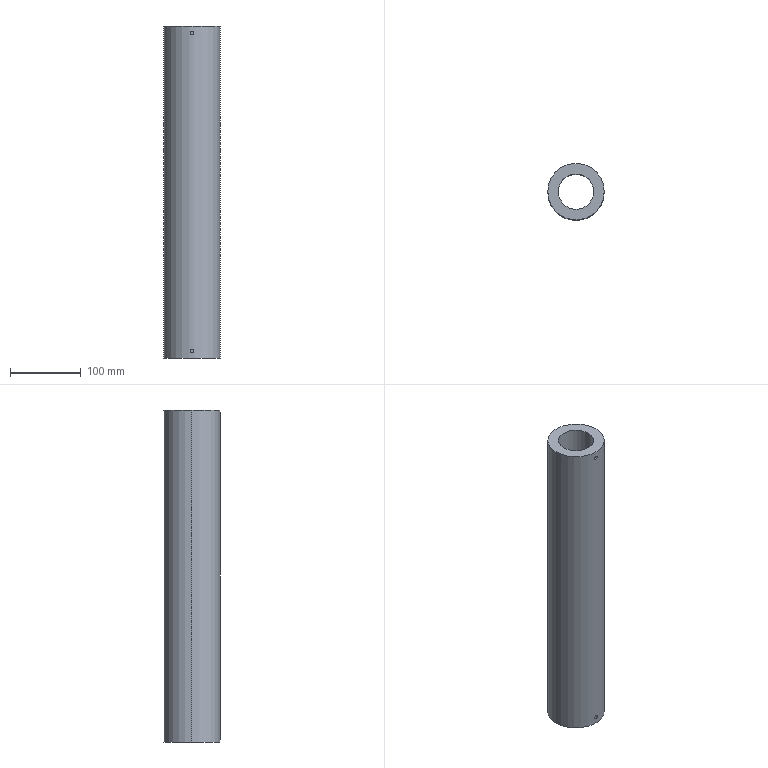Part | SolidWorks | features Extrusion 1, ICE 1 | 1 solid | 10 faces | box 80 x 80 x 470 mm | volume 1439045 mm3 | cylinder 8 | plane 2 | commonest cylinder face diameters 5 x4 50 x2 80 x2
STEP:
#1=CARTESIAN_POINT('',(0.,-40.,462.5));
#2=VERTEX_POINT('',#1);
#3=CARTESIAN_POINT('',(0.,-40.,457.5));
#4=VERTEX_POINT('',#3);
#5=CARTESIAN_POINT('',(0.,-40.,462.5));
#6=CARTESIAN_POINT('',(-0.1652,-40.,462.5));
#7=CARTESIAN_POINT('',(-0.3277,-39.999,462.484));
#8=CARTESIAN_POINT('',(-0.6473,-39.995,462.42));
#9=CARTESIAN_POINT('',(-0.8061,-39.992,462.372));
#10=CARTESIAN_POINT('',(-1.109,-39.985,462.247));
#11=CARTESIAN_POINT('',(-1.252,-39.981,462.17));
#12=CARTESIAN_POINT('',(-1.524,-39.971,461.988));
#13=CARTESIAN_POINT('',(-1.653,-39.966,461.883));
#14=CARTESIAN_POINT('',(-1.883,-39.956,461.652));
#15=CARTESIAN_POINT('',(-1.987,-39.951,461.526));
#16=CARTESIAN_POINT('',(-2.17,-39.941,461.253));
#17=CARTESIAN_POINT('',(-2.247,-39.937,461.107));
#18=CARTESIAN_POINT('',(-2.372,-39.93,460.807));
#19=CARTESIAN_POINT('',(-2.42,-39.927,460.649));
#20=CARTESIAN_POINT('',(-2.484,-39.923,460.326));
#21=CARTESIAN_POINT('',(-2.5,-39.922,460.164));
#22=CARTESIAN_POINT('',(-2.5,-39.922,459.838));
#23=CARTESIAN_POINT('',(-2.484,-39.923,459.672));
#24=CARTESIAN_POINT('',(-2.42,-39.927,459.351));
#25=CARTESIAN_POINT('',(-2.373,-39.93,459.196));
#26=CARTESIAN_POINT('',(-2.247,-39.937,458.893));
#27=CARTESIAN_POINT('',(-2.169,-39.941,458.746));
#28=CARTESIAN_POINT('',(-1.988,-39.951,458.476));
#29=CARTESIAN_POINT('',(-1.885,-39.956,458.349));
#30=CARTESIAN_POINT('',(-1.651,-39.966,458.116));
#31=CARTESIAN_POINT('',(-1.525,-39.971,458.012));
#32=CARTESIAN_POINT('',(-1.254,-39.981,457.831));
#33=CARTESIAN_POINT('',(-1.108,-39.985,457.753));
#34=CARTESIAN_POINT('',(-0.8052,-39.992,457.628));
#35=CARTESIAN_POINT('',(-0.6493,-39.995,457.58));
#36=CARTESIAN_POINT('',(-0.3289,-39.999,457.516));
#37=CARTESIAN_POINT('',(-0.1632,-40.,457.5));
#38=CARTESIAN_POINT('',(0.,-40.,457.5));
#39=B_SPLINE_CURVE_WITH_KNOTS('',3,(#5,#6,#7,#8,#9,#10,#11,#12,#13,#14,#15,#16,#17,#18,#19,#20,#21,#22,#23,#24,#25,#26,#27,#28,#29,#30,#31,#32,#33,#34,#35,#36,#37,#38),.UNSPECIFIED.,.F.,.F.,(4,2,2,2,2,2,2,2,2,2,2,2,2,2,2,2,4),(0.,0.0004886,0.0009773,0.001466,0.001955,0.002443,0.002932,0.00342,0.003909,0.004398,0.004886,0.005375,0.005864,0.006352,0.006841,0.007329,0.007818),.UNSPECIFIED.);
#40=EDGE_CURVE('',#2,#4,#39,.T.);
#41=ORIENTED_EDGE('',*,*,#40,.T.);
#42=CARTESIAN_POINT('',(0.,-25.,457.5));
#43=VERTEX_POINT('',#42);
#44=CARTESIAN_POINT('',(0.,-40.001,457.5));
#45=DIRECTION('',(0.,1.,0.));
#46=VECTOR('',#45,1000.);
#47=LINE('',#44,#46);
#48=EDGE_CURVE('',#4,#43,#47,.T.);
#49=ORIENTED_EDGE('',*,*,#48,.T.);
#50=CARTESIAN_POINT('',(0.,-25.,462.5));
#51=VERTEX_POINT('',#50);
#52=CARTESIAN_POINT('',(0.,-25.,462.5));
#53=CARTESIAN_POINT('',(-0.1653,-25.,462.5));
#54=CARTESIAN_POINT('',(-0.3278,-24.998,462.484));
#55=CARTESIAN_POINT('',(-0.6475,-24.992,462.42));
#56=CARTESIAN_POINT('',(-0.8063,-24.987,462.372));
#57=CARTESIAN_POINT('',(-1.109,-24.976,462.247));
#58=CARTESIAN_POINT('',(-1.253,-24.969,462.17));
#59=CARTESIAN_POINT('',(-1.524,-24.954,461.988));
#60=CARTESIAN_POINT('',(-1.653,-24.946,461.883));
#61=CARTESIAN_POINT('',(-1.883,-24.929,461.652));
#62=CARTESIAN_POINT('',(-1.987,-24.921,461.526));
#63=CARTESIAN_POINT('',(-2.17,-24.906,461.253));
#64=CARTESIAN_POINT('',(-2.247,-24.899,461.108));
#65=CARTESIAN_POINT('',(-2.372,-24.887,460.807));
#66=CARTESIAN_POINT('',(-2.42,-24.883,460.649));
#67=CARTESIAN_POINT('',(-2.484,-24.876,460.326));
#68=CARTESIAN_POINT('',(-2.5,-24.875,460.164));
#69=CARTESIAN_POINT('',(-2.5,-24.875,459.838));
#70=CARTESIAN_POINT('',(-2.484,-24.876,459.672));
#71=CARTESIAN_POINT('',(-2.42,-24.883,459.351));
#72=CARTESIAN_POINT('',(-2.373,-24.887,459.195));
#73=CARTESIAN_POINT('',(-2.247,-24.899,458.893));
#74=CARTESIAN_POINT('',(-2.169,-24.906,458.746));
#75=CARTESIAN_POINT('',(-1.988,-24.921,458.475));
#76=CARTESIAN_POINT('',(-1.885,-24.929,458.349));
#77=CARTESIAN_POINT('',(-1.651,-24.946,458.116));
#78=CARTESIAN_POINT('',(-1.525,-24.954,458.012));
#79=CARTESIAN_POINT('',(-1.254,-24.969,457.831));
#80=CARTESIAN_POINT('',(-1.108,-24.976,457.753));
#81=CARTESIAN_POINT('',(-0.8054,-24.987,457.628));
#82=CARTESIAN_POINT('',(-0.6496,-24.992,457.58));
#83=CARTESIAN_POINT('',(-0.329,-24.998,457.516));
#84=CARTESIAN_POINT('',(-0.1632,-25.,457.5));
#85=CARTESIAN_POINT('',(0.,-25.,457.5));
#86=B_SPLINE_CURVE_WITH_KNOTS('',3,(#52,#53,#54,#55,#56,#57,#58,#59,#60,#61,#62,#63,#64,#65,#66,#67,#68,#69,#70,#71,#72,#73,#74,#75,#76,#77,#78,#79,#80,#81,#82,#83,#84,#85),.UNSPECIFIED.,.F.,.F.,(4,2,2,2,2,2,2,2,2,2,2,2,2,2,2,2,4),(0.,0.0004888,0.0009776,0.001466,0.001955,0.002444,0.002933,0.003422,0.003911,0.004399,0.004888,0.005377,0.005866,0.006355,0.006843,0.007332,0.007821),.UNSPECIFIED.);
#87=EDGE_CURVE('',#51,#43,#86,.T.);
#88=ORIENTED_EDGE('',*,*,#87,.F.);
#89=CARTESIAN_POINT('',(0.,-40.001,462.5));
#90=DIRECTION('',(0.,1.,0.));
#91=VECTOR('',#90,1000.);
#92=LINE('',#89,#91);
#93=EDGE_CURVE('',#2,#51,#92,.T.);
#94=ORIENTED_EDGE('',*,*,#93,.F.);
#95=EDGE_LOOP('',(#41,#49,#88,#94));
#96=FACE_OUTER_BOUND('',#95,.T.);
#97=CARTESIAN_POINT('',(0.,-40.001,460.));
#98=DIRECTION('',(0.,1.,0.));
#99=DIRECTION('',(0.,0.,1.));
#100=AXIS2_PLACEMENT_3D('',#97,#98,#99);
#101=CYLINDRICAL_SURFACE('',#100,2.5);
#102=ADVANCED_FACE('',(#96),#101,.F.);
#103=CARTESIAN_POINT('',(0.,-40.,12.5));
#104=VERTEX_POINT('',#103);
#105=CARTESIAN_POINT('',(0.,-40.,7.5));
#106=VERTEX_POINT('',#105);
#107=CARTESIAN_POINT('',(0.,-40.,12.5));
#108=CARTESIAN_POINT('',(-0.1652,-40.,12.5));
#109=CARTESIAN_POINT('',(-0.3277,-39.999,12.484));
#110=CARTESIAN_POINT('',(-0.6473,-39.995,12.42));
#111=CARTESIAN_POINT('',(-0.8061,-39.992,12.372));
#112=CARTESIAN_POINT('',(-1.109,-39.985,12.247));
#113=CARTESIAN_POINT('',(-1.252,-39.981,12.17));
#114=CARTESIAN_POINT('',(-1.524,-39.971,11.988));
#115=CARTESIAN_POINT('',(-1.653,-39.966,11.883));
#116=CARTESIAN_POINT('',(-1.883,-39.956,11.652));
#117=CARTESIAN_POINT('',(-1.987,-39.951,11.526));
#118=CARTESIAN_POINT('',(-2.17,-39.941,11.253));
#119=CARTESIAN_POINT('',(-2.247,-39.937,11.107));
#120=CARTESIAN_POINT('',(-2.372,-39.93,10.807));
#121=CARTESIAN_POINT('',(-2.42,-39.927,10.649));
#122=CARTESIAN_POINT('',(-2.484,-39.923,10.326));
#123=CARTESIAN_POINT('',(-2.5,-39.922,10.164));
#124=CARTESIAN_POINT('',(-2.5,-39.922,9.838));
#125=CARTESIAN_POINT('',(-2.484,-39.923,9.672));
#126=CARTESIAN_POINT('',(-2.42,-39.927,9.351));
#127=CARTESIAN_POINT('',(-2.373,-39.93,9.196));
#128=CARTESIAN_POINT('',(-2.247,-39.937,8.893));
#129=CARTESIAN_POINT('',(-2.169,-39.941,8.746));
#130=CARTESIAN_POINT('',(-1.988,-39.951,8.476));
#131=CARTESIAN_POINT('',(-1.885,-39.956,8.349));
#132=CARTESIAN_POINT('',(-1.651,-39.966,8.116));
#133=CARTESIAN_POINT('',(-1.525,-39.971,8.012));
#134=CARTESIAN_POINT('',(-1.254,-39.981,7.831));
#135=CARTESIAN_POINT('',(-1.108,-39.985,7.753));
#136=CARTESIAN_POINT('',(-0.8052,-39.992,7.628));
#137=CARTESIAN_POINT('',(-0.6493,-39.995,7.58));
#138=CARTESIAN_POINT('',(-0.3289,-39.999,7.516));
#139=CARTESIAN_POINT('',(-0.1632,-40.,7.5));
#140=CARTESIAN_POINT('',(0.,-40.,7.5));
#141=B_SPLINE_CURVE_WITH_KNOTS('',3,(#107,#108,#109,#110,#111,#112,#113,#114,#115,#116,#117,#118,#119,#120,#121,#122,#123,#124,#125,#126,#127,#128,#129,#130,#131,#132,#133,#134,#135,#136,#137,#138,#139,#140),.UNSPECIFIED.,.F.,.F.,(4,2,2,2,2,2,2,2,2,2,2,2,2,2,2,2,4),(0.,0.0004886,0.0009773,0.001466,0.001955,0.002443,0.002932,0.00342,0.003909,0.004398,0.004886,0.005375,0.005864,0.006352,0.006841,0.007329,0.007818),.UNSPECIFIED.);
#142=EDGE_CURVE('',#104,#106,#141,.T.);
#143=ORIENTED_EDGE('',*,*,#142,.T.);
#144=CARTESIAN_POINT('',(0.,-25.,7.5));
#145=VERTEX_POINT('',#144);
#146=CARTESIAN_POINT('',(0.,-40.001,7.5));
#147=DIRECTION('',(0.,1.,0.));
#148=VECTOR('',#147,1000.);
#149=LINE('',#146,#148);
#150=EDGE_CURVE('',#106,#145,#149,.T.);
#151=ORIENTED_EDGE('',*,*,#150,.T.);
#152=CARTESIAN_POINT('',(0.,-25.,12.5));
#153=VERTEX_POINT('',#152);
#154=CARTESIAN_POINT('',(0.,-25.,12.5));
#155=CARTESIAN_POINT('',(-0.1653,-25.,12.5));
#156=CARTESIAN_POINT('',(-0.3278,-24.998,12.484));
#157=CARTESIAN_POINT('',(-0.6475,-24.992,12.42));
#158=CARTESIAN_POINT('',(-0.8063,-24.987,12.372));
#159=CARTESIAN_POINT('',(-1.109,-24.976,12.247));
#160=CARTESIAN_POINT('',(-1.253,-24.969,12.17));
#161=CARTESIAN_POINT('',(-1.524,-24.954,11.988));
#162=CARTESIAN_POINT('',(-1.653,-24.946,11.883));
#163=CARTESIAN_POINT('',(-1.883,-24.929,11.652));
#164=CARTESIAN_POINT('',(-1.987,-24.921,11.526));
#165=CARTESIAN_POINT('',(-2.17,-24.906,11.253));
#166=CARTESIAN_POINT('',(-2.247,-24.899,11.108));
#167=CARTESIAN_POINT('',(-2.372,-24.887,10.807));
#168=CARTESIAN_POINT('',(-2.42,-24.883,10.649));
#169=CARTESIAN_POINT('',(-2.484,-24.876,10.326));
#170=CARTESIAN_POINT('',(-2.5,-24.875,10.164));
#171=CARTESIAN_POINT('',(-2.5,-24.875,9.838));
#172=CARTESIAN_POINT('',(-2.484,-24.876,9.672));
#173=CARTESIAN_POINT('',(-2.42,-24.883,9.351));
#174=CARTESIAN_POINT('',(-2.373,-24.887,9.195));
#175=CARTESIAN_POINT('',(-2.247,-24.899,8.893));
#176=CARTESIAN_POINT('',(-2.169,-24.906,8.746));
#177=CARTESIAN_POINT('',(-1.988,-24.921,8.475));
#178=CARTESIAN_POINT('',(-1.885,-24.929,8.349));
#179=CARTESIAN_POINT('',(-1.651,-24.946,8.116));
#180=CARTESIAN_POINT('',(-1.525,-24.954,8.012));
#181=CARTESIAN_POINT('',(-1.254,-24.969,7.831));
#182=CARTESIAN_POINT('',(-1.108,-24.976,7.753));
#183=CARTESIAN_POINT('',(-0.8054,-24.987,7.628));
#184=CARTESIAN_POINT('',(-0.6496,-24.992,7.58));
#185=CARTESIAN_POINT('',(-0.329,-24.998,7.516));
#186=CARTESIAN_POINT('',(-0.1632,-25.,7.5));
#187=CARTESIAN_POINT('',(0.,-25.,7.5));
#188=B_SPLINE_CURVE_WITH_KNOTS('',3,(#154,#155,#156,#157,#158,#159,#160,#161,#162,#163,#164,#165,#166,#167,#168,#169,#170,#171,#172,#173,#174,#175,#176,#177,#178,#179,#180,#181,#182,#183,#184,#185,#186,#187),.UNSPECIFIED.,.F.,.F.,(4,2,2,2,2,2,2,2,2,2,2,2,2,2,2,2,4),(0.,0.0004888,0.0009776,0.001466,0.001955,0.002444,0.002933,0.003422,0.003911,0.004399,0.004888,0.005377,0.005866,0.006355,0.006843,0.007332,0.007821),.UNSPECIFIED.);
#189=EDGE_CURVE('',#153,#145,#188,.T.);
#190=ORIENTED_EDGE('',*,*,#189,.F.);
#191=CARTESIAN_POINT('',(0.,-40.001,12.5));
#192=DIRECTION('',(0.,1.,0.));
#193=VECTOR('',#192,1000.);
#194=LINE('',#191,#193);
#195=EDGE_CURVE('',#104,#153,#194,.T.);
#196=ORIENTED_EDGE('',*,*,#195,.F.);
#197=EDGE_LOOP('',(#143,#151,#190,#196));
#198=FACE_OUTER_BOUND('',#197,.T.);
#199=CARTESIAN_POINT('',(0.,-40.001,10.));
#200=DIRECTION('',(0.,1.,0.));
#201=DIRECTION('',(0.,0.,1.));
#202=AXIS2_PLACEMENT_3D('',#199,#200,#201);
#203=CYLINDRICAL_SURFACE('',#202,2.5);
#204=ADVANCED_FACE('',(#198),#203,.F.);
#205=ORIENTED_EDGE('',*,*,#87,.T.);
#206=CARTESIAN_POINT('',(0.,-25.,457.5));
#207=CARTESIAN_POINT('',(0.1632,-25.,457.5));
#208=CARTESIAN_POINT('',(0.3254,-24.998,457.516));
#209=CARTESIAN_POINT('',(0.648,-24.992,457.58));
#210=CARTESIAN_POINT('',(0.8058,-24.987,457.628));
#211=CARTESIAN_POINT('',(1.107,-24.976,457.752));
#212=CARTESIAN_POINT('',(1.252,-24.969,457.83));
#213=CARTESIAN_POINT('',(1.525,-24.954,458.013));
#214=CARTESIAN_POINT('',(1.651,-24.946,458.116));
#215=CARTESIAN_POINT('',(1.882,-24.929,458.346));
#216=CARTESIAN_POINT('',(1.987,-24.921,458.475));
#217=CARTESIAN_POINT('',(2.169,-24.906,458.746));
#218=CARTESIAN_POINT('',(2.246,-24.899,458.89));
#219=CARTESIAN_POINT('',(2.372,-24.887,459.192));
#220=CARTESIAN_POINT('',(2.42,-24.883,459.351));
#221=CARTESIAN_POINT('',(2.484,-24.876,459.671));
#222=CARTESIAN_POINT('',(2.5,-24.875,459.833));
#223=CARTESIAN_POINT('',(2.5,-24.875,460.163));
#224=CARTESIAN_POINT('',(2.484,-24.876,460.326));
#225=CARTESIAN_POINT('',(2.421,-24.883,460.646));
#226=CARTESIAN_POINT('',(2.373,-24.887,460.804));
#227=CARTESIAN_POINT('',(2.247,-24.899,461.107));
#228=CARTESIAN_POINT('',(2.171,-24.906,461.251));
#229=CARTESIAN_POINT('',(1.99,-24.921,461.523));
#230=CARTESIAN_POINT('',(1.884,-24.929,461.651));
#231=CARTESIAN_POINT('',(1.654,-24.946,461.882));
#232=CARTESIAN_POINT('',(1.528,-24.954,461.985));
#233=CARTESIAN_POINT('',(1.255,-24.969,462.168));
#234=CARTESIAN_POINT('',(1.11,-24.976,462.246));
#235=CARTESIAN_POINT('',(0.6589,-24.993,462.433));
#236=CARTESIAN_POINT('',(0.3305,-25.,462.5));
#237=CARTESIAN_POINT('',(0.,-25.,462.5));
#238=B_SPLINE_CURVE_WITH_KNOTS('',3,(#206,#207,#208,#209,#210,#211,#212,#213,#214,#215,#216,#217,#218,#219,#220,#221,#222,#223,#224,#225,#226,#227,#228,#229,#230,#231,#232,#233,#234,#235,#236,#237),.UNSPECIFIED.,.F.,.F.,(4,2,2,2,2,2,2,2,2,2,2,2,2,2,2,4),(0.007821,0.00831,0.008798,0.009287,0.009776,0.01026,0.01075,0.01124,0.01173,0.01222,0.01271,0.0132,0.01369,0.01417,0.01466,0.01564),.UNSPECIFIED.);
#239=EDGE_CURVE('',#43,#51,#238,.T.);
#240=ORIENTED_EDGE('',*,*,#239,.T.);
#241=EDGE_LOOP('',(#205,#240));
#242=FACE_BOUND('',#241,.T.);
#243=ORIENTED_EDGE('',*,*,#189,.T.);
#244=CARTESIAN_POINT('',(0.,-25.,7.5));
#245=CARTESIAN_POINT('',(0.1632,-25.,7.5));
#246=CARTESIAN_POINT('',(0.3254,-24.998,7.516));
#247=CARTESIAN_POINT('',(0.648,-24.992,7.58));
#248=CARTESIAN_POINT('',(0.8058,-24.987,7.628));
#249=CARTESIAN_POINT('',(1.107,-24.976,7.752));
#250=CARTESIAN_POINT('',(1.252,-24.969,7.83));
#251=CARTESIAN_POINT('',(1.525,-24.954,8.013));
#252=CARTESIAN_POINT('',(1.651,-24.946,8.116));
#253=CARTESIAN_POINT('',(1.882,-24.929,8.346));
#254=CARTESIAN_POINT('',(1.987,-24.921,8.475));
#255=CARTESIAN_POINT('',(2.169,-24.906,8.746));
#256=CARTESIAN_POINT('',(2.246,-24.899,8.89));
#257=CARTESIAN_POINT('',(2.372,-24.887,9.192));
#258=CARTESIAN_POINT('',(2.42,-24.883,9.351));
#259=CARTESIAN_POINT('',(2.484,-24.876,9.671));
#260=CARTESIAN_POINT('',(2.5,-24.875,9.833));
#261=CARTESIAN_POINT('',(2.5,-24.875,10.163));
#262=CARTESIAN_POINT('',(2.484,-24.876,10.326));
#263=CARTESIAN_POINT('',(2.421,-24.883,10.646));
#264=CARTESIAN_POINT('',(2.373,-24.887,10.804));
#265=CARTESIAN_POINT('',(2.247,-24.899,11.107));
#266=CARTESIAN_POINT('',(2.171,-24.906,11.251));
#267=CARTESIAN_POINT('',(1.99,-24.921,11.523));
#268=CARTESIAN_POINT('',(1.884,-24.929,11.651));
#269=CARTESIAN_POINT('',(1.654,-24.946,11.882));
#270=CARTESIAN_POINT('',(1.528,-24.954,11.985));
#271=CARTESIAN_POINT('',(1.255,-24.969,12.168));
#272=CARTESIAN_POINT('',(1.11,-24.976,12.246));
#273=CARTESIAN_POINT('',(0.6589,-24.993,12.433));
#274=CARTESIAN_POINT('',(0.3305,-25.,12.5));
#275=CARTESIAN_POINT('',(0.,-25.,12.5));
#276=B_SPLINE_CURVE_WITH_KNOTS('',3,(#244,#245,#246,#247,#248,#249,#250,#251,#252,#253,#254,#255,#256,#257,#258,#259,#260,#261,#262,#263,#264,#265,#266,#267,#268,#269,#270,#271,#272,#273,#274,#275),.UNSPECIFIED.,.F.,.F.,(4,2,2,2,2,2,2,2,2,2,2,2,2,2,2,4),(0.007821,0.00831,0.008798,0.009287,0.009776,0.01026,0.01075,0.01124,0.01173,0.01222,0.01271,0.0132,0.01369,0.01417,0.01466,0.01564),.UNSPECIFIED.);
#277=EDGE_CURVE('',#145,#153,#276,.T.);
#278=ORIENTED_EDGE('',*,*,#277,.T.);
#279=EDGE_LOOP('',(#243,#278));
#280=FACE_BOUND('',#279,.T.);
#281=CARTESIAN_POINT('',(-25.,0.,470.));
#282=VERTEX_POINT('',#281);
#283=CARTESIAN_POINT('',(25.,0.,470.));
#284=VERTEX_POINT('',#283);
#285=CARTESIAN_POINT('',(0.,0.,470.));
#286=DIRECTION('',(0.,0.,1.));
#287=DIRECTION('',(1.,0.,0.));
#288=AXIS2_PLACEMENT_3D('',#285,#286,#287);
#289=CIRCLE('',#288,25.);
#290=EDGE_CURVE('',#282,#284,#289,.T.);
#291=ORIENTED_EDGE('',*,*,#290,.T.);
#292=CARTESIAN_POINT('',(25.,0.,0.));
#293=VERTEX_POINT('',#292);
#294=CARTESIAN_POINT('',(25.,0.,470.));
#295=DIRECTION('',(0.,0.,-1.));
#296=VECTOR('',#295,1000.);
#297=LINE('',#294,#296);
#298=EDGE_CURVE('',#284,#293,#297,.T.);
#299=ORIENTED_EDGE('',*,*,#298,.T.);
#300=CARTESIAN_POINT('',(-25.,0.,0.));
#301=VERTEX_POINT('',#300);
#302=CARTESIAN_POINT('',(0.,0.,0.));
#303=DIRECTION('',(0.,0.,1.));
#304=DIRECTION('',(1.,0.,0.));
#305=AXIS2_PLACEMENT_3D('',#302,#303,#304);
#306=CIRCLE('',#305,25.);
#307=EDGE_CURVE('',#301,#293,#306,.T.);
#308=ORIENTED_EDGE('',*,*,#307,.F.);
#309=CARTESIAN_POINT('',(-25.,0.,470.));
#310=DIRECTION('',(0.,0.,-1.));
#311=VECTOR('',#310,1000.);
#312=LINE('',#309,#311);
#313=EDGE_CURVE('',#282,#301,#312,.T.);
#314=ORIENTED_EDGE('',*,*,#313,.F.);
#315=EDGE_LOOP('',(#291,#299,#308,#314));
#316=FACE_OUTER_BOUND('',#315,.T.);
#317=CARTESIAN_POINT('',(0.,0.,470.));
#318=DIRECTION('',(0.,0.,-1.));
#319=DIRECTION('',(-1.,0.,0.));
#320=AXIS2_PLACEMENT_3D('',#317,#318,#319);
#321=CYLINDRICAL_SURFACE('',#320,25.);
#322=ADVANCED_FACE('',(#242,#280,#316),#321,.F.);
#323=CARTESIAN_POINT('',(40.,0.,470.));
#324=VERTEX_POINT('',#323);
#325=CARTESIAN_POINT('',(-40.,0.,470.));
#326=VERTEX_POINT('',#325);
#327=CARTESIAN_POINT('',(0.,0.,470.));
#328=DIRECTION('',(0.,0.,1.));
#329=DIRECTION('',(1.,0.,0.));
#330=AXIS2_PLACEMENT_3D('',#327,#328,#329);
#331=CIRCLE('',#330,40.);
#332=EDGE_CURVE('',#324,#326,#331,.T.);
#333=ORIENTED_EDGE('',*,*,#332,.F.);
#334=CARTESIAN_POINT('',(40.,0.,0.));
#335=VERTEX_POINT('',#334);
#336=CARTESIAN_POINT('',(40.,0.,470.));
#337=DIRECTION('',(0.,0.,-1.));
#338=VECTOR('',#337,1000.);
#339=LINE('',#336,#338);
#340=EDGE_CURVE('',#324,#335,#339,.T.);
#341=ORIENTED_EDGE('',*,*,#340,.T.);
#342=CARTESIAN_POINT('',(-40.,0.,0.));
#343=VERTEX_POINT('',#342);
#344=CARTESIAN_POINT('',(0.,0.,0.));
#345=DIRECTION('',(0.,0.,1.));
#346=DIRECTION('',(1.,0.,0.));
#347=AXIS2_PLACEMENT_3D('',#344,#345,#346);
#348=CIRCLE('',#347,40.);
#349=EDGE_CURVE('',#335,#343,#348,.T.);
#350=ORIENTED_EDGE('',*,*,#349,.T.);
#351=CARTESIAN_POINT('',(-40.,0.,470.));
#352=DIRECTION('',(0.,0.,-1.));
#353=VECTOR('',#352,1000.);
#354=LINE('',#351,#353);
#355=EDGE_CURVE('',#326,#343,#354,.T.);
#356=ORIENTED_EDGE('',*,*,#355,.F.);
#357=EDGE_LOOP('',(#333,#341,#350,#356));
#358=FACE_OUTER_BOUND('',#357,.T.);
#359=CARTESIAN_POINT('',(0.,0.,470.));
#360=DIRECTION('',(0.,0.,-1.));
#361=DIRECTION('',(-1.,0.,0.));
#362=AXIS2_PLACEMENT_3D('',#359,#360,#361);
#363=CYLINDRICAL_SURFACE('',#362,40.);
#364=ADVANCED_FACE('',(#358),#363,.T.);
#365=CARTESIAN_POINT('',(0.,0.,470.));
#366=DIRECTION('',(0.,0.,1.));
#367=DIRECTION('',(1.,0.,0.));
#368=AXIS2_PLACEMENT_3D('',#365,#366,#367);
#369=CIRCLE('',#368,40.);
#370=EDGE_CURVE('',#326,#324,#369,.T.);
#371=ORIENTED_EDGE('',*,*,#370,.T.);
#372=ORIENTED_EDGE('',*,*,#332,.T.);
#373=EDGE_LOOP('',(#371,#372));
#374=FACE_OUTER_BOUND('',#373,.T.);
#375=ORIENTED_EDGE('',*,*,#290,.F.);
#376=CARTESIAN_POINT('',(0.,0.,470.));
#377=DIRECTION('',(0.,0.,1.));
#378=DIRECTION('',(1.,0.,0.));
#379=AXIS2_PLACEMENT_3D('',#376,#377,#378);
#380=CIRCLE('',#379,25.);
#381=EDGE_CURVE('',#284,#282,#380,.T.);
#382=ORIENTED_EDGE('',*,*,#381,.F.);
#383=EDGE_LOOP('',(#375,#382));
#384=FACE_BOUND('',#383,.T.);
#385=CARTESIAN_POINT('',(0.,0.,470.));
#386=DIRECTION('',(0.,0.,1.));
#387=DIRECTION('',(1.,0.,0.));
#388=AXIS2_PLACEMENT_3D('',#385,#386,#387);
#389=PLANE('',#388);
#390=ADVANCED_FACE('',(#374,#384),#389,.T.);
#391=CARTESIAN_POINT('',(0.,0.,0.));
#392=DIRECTION('',(0.,0.,1.));
#393=DIRECTION('',(1.,0.,0.));
#394=AXIS2_PLACEMENT_3D('',#391,#392,#393);
#395=CIRCLE('',#394,40.);
#396=EDGE_CURVE('',#343,#335,#395,.T.);
#397=ORIENTED_EDGE('',*,*,#396,.F.);
#398=ORIENTED_EDGE('',*,*,#349,.F.);
#399=EDGE_LOOP('',(#397,#398));
#400=FACE_OUTER_BOUND('',#399,.T.);
#401=ORIENTED_EDGE('',*,*,#307,.T.);
#402=CARTESIAN_POINT('',(0.,0.,0.));
#403=DIRECTION('',(0.,0.,1.));
#404=DIRECTION('',(1.,0.,0.));
#405=AXIS2_PLACEMENT_3D('',#402,#403,#404);
#406=CIRCLE('',#405,25.);
#407=EDGE_CURVE('',#293,#301,#406,.T.);
#408=ORIENTED_EDGE('',*,*,#407,.T.);
#409=EDGE_LOOP('',(#401,#408));
#410=FACE_BOUND('',#409,.T.);
#411=CARTESIAN_POINT('',(0.,0.,0.));
#412=DIRECTION('',(0.,0.,1.));
#413=DIRECTION('',(1.,0.,0.));
#414=AXIS2_PLACEMENT_3D('',#411,#412,#413);
#415=PLANE('',#414);
#416=ADVANCED_FACE('',(#400,#410),#415,.F.);
#417=ORIENTED_EDGE('',*,*,#340,.F.);
#418=ORIENTED_EDGE('',*,*,#370,.F.);
#419=ORIENTED_EDGE('',*,*,#355,.T.);
#420=ORIENTED_EDGE('',*,*,#396,.T.);
#421=EDGE_LOOP('',(#417,#418,#419,#420));
#422=FACE_OUTER_BOUND('',#421,.T.);
#423=ORIENTED_EDGE('',*,*,#40,.F.);
#424=CARTESIAN_POINT('',(0.,-40.,457.5));
#425=CARTESIAN_POINT('',(0.1631,-40.,457.5));
#426=CARTESIAN_POINT('',(0.3253,-39.999,457.516));
#427=CARTESIAN_POINT('',(0.6477,-39.995,457.58));
#428=CARTESIAN_POINT('',(0.8056,-39.992,457.628));
#429=CARTESIAN_POINT('',(1.257,-39.981,457.815));
#430=CARTESIAN_POINT('',(1.536,-39.971,458.001));
#431=CARTESIAN_POINT('',(1.882,-39.956,458.346));
#432=CARTESIAN_POINT('',(1.987,-39.951,458.475));
#433=CARTESIAN_POINT('',(2.169,-39.941,458.746));
#434=CARTESIAN_POINT('',(2.246,-39.937,458.89));
#435=CARTESIAN_POINT('',(2.372,-39.93,459.192));
#436=CARTESIAN_POINT('',(2.42,-39.927,459.351));
#437=CARTESIAN_POINT('',(2.484,-39.923,459.671));
#438=CARTESIAN_POINT('',(2.5,-39.922,459.833));
#439=CARTESIAN_POINT('',(2.5,-39.922,460.163));
#440=CARTESIAN_POINT('',(2.484,-39.923,460.326));
#441=CARTESIAN_POINT('',(2.421,-39.927,460.645));
#442=CARTESIAN_POINT('',(2.373,-39.93,460.804));
#443=CARTESIAN_POINT('',(2.248,-39.937,461.107));
#444=CARTESIAN_POINT('',(2.171,-39.941,461.251));
#445=CARTESIAN_POINT('',(1.99,-39.951,461.522));
#446=CARTESIAN_POINT('',(1.884,-39.956,461.651));
#447=CARTESIAN_POINT('',(1.654,-39.966,461.882));
#448=CARTESIAN_POINT('',(1.528,-39.971,461.985));
#449=CARTESIAN_POINT('',(1.255,-39.981,462.168));
#450=CARTESIAN_POINT('',(1.11,-39.985,462.246));
#451=CARTESIAN_POINT('',(0.6586,-39.996,462.434));
#452=CARTESIAN_POINT('',(0.3304,-40.,462.5));
#453=CARTESIAN_POINT('',(0.,-40.,462.5));
#454=B_SPLINE_CURVE_WITH_KNOTS('',3,(#424,#425,#426,#427,#428,#429,#430,#431,#432,#433,#434,#435,#436,#437,#438,#439,#440,#441,#442,#443,#444,#445,#446,#447,#448,#449,#450,#451,#452,#453),.UNSPECIFIED.,.F.,.F.,(4,2,2,2,2,2,2,2,2,2,2,2,2,2,4),(0.007818,0.008307,0.008795,0.009772,0.01026,0.01075,0.01124,0.01173,0.01221,0.0127,0.01319,0.01368,0.01417,0.01466,0.01563),.UNSPECIFIED.);
#455=EDGE_CURVE('',#4,#2,#454,.T.);
#456=ORIENTED_EDGE('',*,*,#455,.F.);
#457=EDGE_LOOP('',(#423,#456));
#458=FACE_BOUND('',#457,.T.);
#459=ORIENTED_EDGE('',*,*,#142,.F.);
#460=CARTESIAN_POINT('',(0.,-40.,7.5));
#461=CARTESIAN_POINT('',(0.1631,-40.,7.5));
#462=CARTESIAN_POINT('',(0.3253,-39.999,7.516));
#463=CARTESIAN_POINT('',(0.6477,-39.995,7.58));
#464=CARTESIAN_POINT('',(0.8056,-39.992,7.628));
#465=CARTESIAN_POINT('',(1.257,-39.981,7.815));
#466=CARTESIAN_POINT('',(1.536,-39.971,8.001));
#467=CARTESIAN_POINT('',(1.882,-39.956,8.346));
#468=CARTESIAN_POINT('',(1.987,-39.951,8.475));
#469=CARTESIAN_POINT('',(2.169,-39.941,8.746));
#470=CARTESIAN_POINT('',(2.246,-39.937,8.89));
#471=CARTESIAN_POINT('',(2.372,-39.93,9.192));
#472=CARTESIAN_POINT('',(2.42,-39.927,9.351));
#473=CARTESIAN_POINT('',(2.484,-39.923,9.671));
#474=CARTESIAN_POINT('',(2.5,-39.922,9.833));
#475=CARTESIAN_POINT('',(2.5,-39.922,10.163));
#476=CARTESIAN_POINT('',(2.484,-39.923,10.326));
#477=CARTESIAN_POINT('',(2.421,-39.927,10.645));
#478=CARTESIAN_POINT('',(2.373,-39.93,10.804));
#479=CARTESIAN_POINT('',(2.248,-39.937,11.107));
#480=CARTESIAN_POINT('',(2.171,-39.941,11.251));
#481=CARTESIAN_POINT('',(1.99,-39.951,11.522));
#482=CARTESIAN_POINT('',(1.884,-39.956,11.651));
#483=CARTESIAN_POINT('',(1.654,-39.966,11.882));
#484=CARTESIAN_POINT('',(1.528,-39.971,11.985));
#485=CARTESIAN_POINT('',(1.255,-39.981,12.168));
#486=CARTESIAN_POINT('',(1.11,-39.985,12.246));
#487=CARTESIAN_POINT('',(0.6586,-39.996,12.434));
#488=CARTESIAN_POINT('',(0.3304,-40.,12.5));
#489=CARTESIAN_POINT('',(0.,-40.,12.5));
#490=B_SPLINE_CURVE_WITH_KNOTS('',3,(#460,#461,#462,#463,#464,#465,#466,#467,#468,#469,#470,#471,#472,#473,#474,#475,#476,#477,#478,#479,#480,#481,#482,#483,#484,#485,#486,#487,#488,#489),.UNSPECIFIED.,.F.,.F.,(4,2,2,2,2,2,2,2,2,2,2,2,2,2,4),(0.007818,0.008307,0.008795,0.009772,0.01026,0.01075,0.01124,0.01173,0.01221,0.0127,0.01319,0.01368,0.01417,0.01466,0.01563),.UNSPECIFIED.);
#491=EDGE_CURVE('',#106,#104,#490,.T.);
#492=ORIENTED_EDGE('',*,*,#491,.F.);
#493=EDGE_LOOP('',(#459,#492));
#494=FACE_BOUND('',#493,.T.);
#495=CARTESIAN_POINT('',(0.,0.,470.));
#496=DIRECTION('',(0.,0.,-1.));
#497=DIRECTION('',(-1.,0.,0.));
#498=AXIS2_PLACEMENT_3D('',#495,#496,#497);
#499=CYLINDRICAL_SURFACE('',#498,40.);
#500=ADVANCED_FACE('',(#422,#458,#494),#499,.T.);
#501=ORIENTED_EDGE('',*,*,#298,.F.);
#502=ORIENTED_EDGE('',*,*,#381,.T.);
#503=ORIENTED_EDGE('',*,*,#313,.T.);
#504=ORIENTED_EDGE('',*,*,#407,.F.);
#505=EDGE_LOOP('',(#501,#502,#503,#504));
#506=FACE_OUTER_BOUND('',#505,.T.);
#507=CARTESIAN_POINT('',(0.,0.,470.));
#508=DIRECTION('',(0.,0.,-1.));
#509=DIRECTION('',(-1.,0.,0.));
#510=AXIS2_PLACEMENT_3D('',#507,#508,#509);
#511=CYLINDRICAL_SURFACE('',#510,25.);
#512=ADVANCED_FACE('',(#506),#511,.F.);
#513=ORIENTED_EDGE('',*,*,#150,.F.);
#514=ORIENTED_EDGE('',*,*,#491,.T.);
#515=ORIENTED_EDGE('',*,*,#195,.T.);
#516=ORIENTED_EDGE('',*,*,#277,.F.);
#517=EDGE_LOOP('',(#513,#514,#515,#516));
#518=FACE_OUTER_BOUND('',#517,.T.);
#519=CARTESIAN_POINT('',(0.,-40.001,10.));
#520=DIRECTION('',(0.,1.,0.));
#521=DIRECTION('',(0.,0.,1.));
#522=AXIS2_PLACEMENT_3D('',#519,#520,#521);
#523=CYLINDRICAL_SURFACE('',#522,2.5);
#524=ADVANCED_FACE('',(#518),#523,.F.);
#525=ORIENTED_EDGE('',*,*,#48,.F.);
#526=ORIENTED_EDGE('',*,*,#455,.T.);
#527=ORIENTED_EDGE('',*,*,#93,.T.);
#528=ORIENTED_EDGE('',*,*,#239,.F.);
#529=EDGE_LOOP('',(#525,#526,#527,#528));
#530=FACE_OUTER_BOUND('',#529,.T.);
#531=CARTESIAN_POINT('',(0.,-40.001,460.));
#532=DIRECTION('',(0.,1.,0.));
#533=DIRECTION('',(0.,0.,1.));
#534=AXIS2_PLACEMENT_3D('',#531,#532,#533);
#535=CYLINDRICAL_SURFACE('',#534,2.5);
#536=ADVANCED_FACE('',(#530),#535,.F.);
#537=CLOSED_SHELL('',(#102,#204,#322,#364,#390,#416,#500,#512,#524,#536));
#538=MANIFOLD_SOLID_BREP('',#537);
#539=CARTESIAN_POINT('',(0.,0.,0.));
#540=DIRECTION('',(0.,0.,1.));
#541=DIRECTION('',(1.,0.,0.));
#542=AXIS2_PLACEMENT_3D('',#539,#540,#541);
#543=(LENGTH_UNIT()NAMED_UNIT(*)SI_UNIT(.MILLI.,.METRE.));
#544=UNCERTAINTY_MEASURE_WITH_UNIT(LENGTH_MEASURE(0.00001),#543,'','');
#545=(NAMED_UNIT(*)PLANE_ANGLE_UNIT()SI_UNIT($,.RADIAN.));
#546=(NAMED_UNIT(*)SI_UNIT($,.STERADIAN.)SOLID_ANGLE_UNIT());
#547=(GEOMETRIC_REPRESENTATION_CONTEXT(3)GLOBAL_UNCERTAINTY_ASSIGNED_CONTEXT((#544))GLOBAL_UNIT_ASSIGNED_CONTEXT((#543,#545,#546))REPRESENTATION_CONTEXT('',''));
#548=ADVANCED_BREP_SHAPE_REPRESENTATION('',(#538,#542),#547);